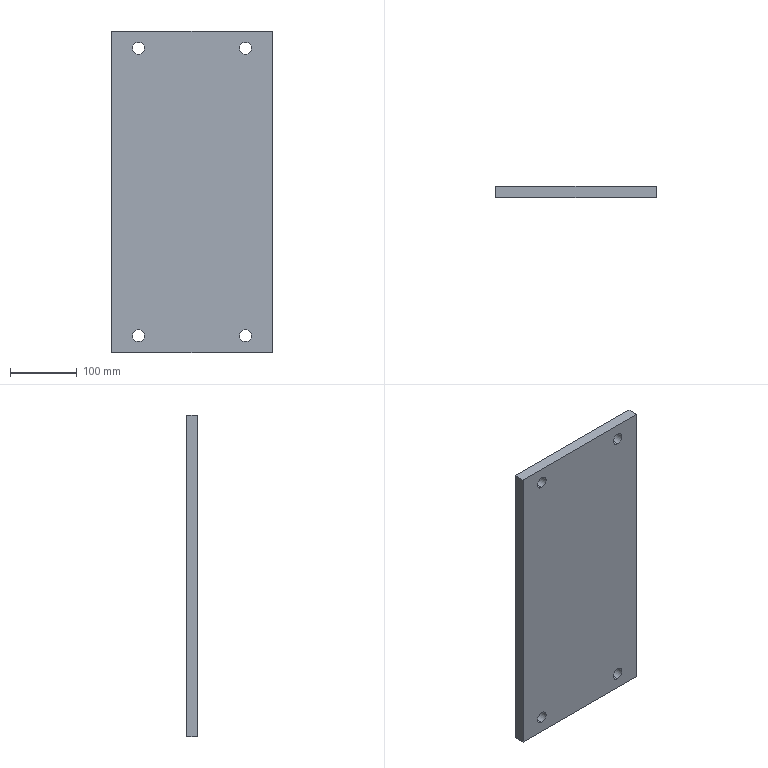Part | SolidWorks | features Chamfer 1, Extrusion 1, Fillet 1, HoleWzd 1 | 1 solid | 14 faces | box 240 x 16 x 480 mm | volume 1826914 mm3 | cylinder 8 | plane 6 | commonest cylinder face diameters 18 x8
STEP:
#1=CARTESIAN_POINT('',(-80.,0.,206.));
#2=VERTEX_POINT('',#1);
#3=CARTESIAN_POINT('',(-80.,0.,224.));
#4=VERTEX_POINT('',#3);
#5=CARTESIAN_POINT('',(-80.,0.,215.));
#6=DIRECTION('',(0.,1.,0.));
#7=DIRECTION('',(0.,0.,1.));
#8=AXIS2_PLACEMENT_3D('',#5,#6,#7);
#9=CIRCLE('',#8,9.);
#10=EDGE_CURVE('',#2,#4,#9,.T.);
#11=ORIENTED_EDGE('',*,*,#10,.F.);
#12=CARTESIAN_POINT('',(-80.,16.,206.));
#13=VERTEX_POINT('',#12);
#14=CARTESIAN_POINT('',(-80.,16.,206.));
#15=DIRECTION('',(0.,1.,0.));
#16=VECTOR('',#15,1000.);
#17=LINE('',#14,#16);
#18=EDGE_CURVE('',#2,#13,#17,.T.);
#19=ORIENTED_EDGE('',*,*,#18,.T.);
#20=CARTESIAN_POINT('',(-80.,16.,224.));
#21=VERTEX_POINT('',#20);
#22=CARTESIAN_POINT('',(-80.,16.,215.));
#23=DIRECTION('',(0.,1.,0.));
#24=DIRECTION('',(0.,0.,1.));
#25=AXIS2_PLACEMENT_3D('',#22,#23,#24);
#26=CIRCLE('',#25,9.);
#27=EDGE_CURVE('',#13,#21,#26,.T.);
#28=ORIENTED_EDGE('',*,*,#27,.T.);
#29=CARTESIAN_POINT('',(-80.,16.,224.));
#30=DIRECTION('',(0.,1.,0.));
#31=VECTOR('',#30,1000.);
#32=LINE('',#29,#31);
#33=EDGE_CURVE('',#4,#21,#32,.T.);
#34=ORIENTED_EDGE('',*,*,#33,.F.);
#35=EDGE_LOOP('',(#11,#19,#28,#34));
#36=FACE_OUTER_BOUND('',#35,.T.);
#37=CARTESIAN_POINT('',(-80.,16.,215.));
#38=DIRECTION('',(0.,1.,0.));
#39=DIRECTION('',(0.,0.,1.));
#40=AXIS2_PLACEMENT_3D('',#37,#38,#39);
#41=CYLINDRICAL_SURFACE('',#40,9.);
#42=ADVANCED_FACE('',(#36),#41,.F.);
#43=CARTESIAN_POINT('',(80.,0.,206.));
#44=VERTEX_POINT('',#43);
#45=CARTESIAN_POINT('',(80.,0.,224.));
#46=VERTEX_POINT('',#45);
#47=CARTESIAN_POINT('',(80.,0.,215.));
#48=DIRECTION('',(0.,1.,0.));
#49=DIRECTION('',(0.,0.,1.));
#50=AXIS2_PLACEMENT_3D('',#47,#48,#49);
#51=CIRCLE('',#50,9.);
#52=EDGE_CURVE('',#44,#46,#51,.T.);
#53=ORIENTED_EDGE('',*,*,#52,.F.);
#54=CARTESIAN_POINT('',(80.,16.,206.));
#55=VERTEX_POINT('',#54);
#56=CARTESIAN_POINT('',(80.,16.,206.));
#57=DIRECTION('',(0.,1.,0.));
#58=VECTOR('',#57,1000.);
#59=LINE('',#56,#58);
#60=EDGE_CURVE('',#44,#55,#59,.T.);
#61=ORIENTED_EDGE('',*,*,#60,.T.);
#62=CARTESIAN_POINT('',(80.,16.,224.));
#63=VERTEX_POINT('',#62);
#64=CARTESIAN_POINT('',(80.,16.,215.));
#65=DIRECTION('',(0.,1.,0.));
#66=DIRECTION('',(0.,0.,1.));
#67=AXIS2_PLACEMENT_3D('',#64,#65,#66);
#68=CIRCLE('',#67,9.);
#69=EDGE_CURVE('',#55,#63,#68,.T.);
#70=ORIENTED_EDGE('',*,*,#69,.T.);
#71=CARTESIAN_POINT('',(80.,16.,224.));
#72=DIRECTION('',(0.,1.,0.));
#73=VECTOR('',#72,1000.);
#74=LINE('',#71,#73);
#75=EDGE_CURVE('',#46,#63,#74,.T.);
#76=ORIENTED_EDGE('',*,*,#75,.F.);
#77=EDGE_LOOP('',(#53,#61,#70,#76));
#78=FACE_OUTER_BOUND('',#77,.T.);
#79=CARTESIAN_POINT('',(80.,16.,215.));
#80=DIRECTION('',(0.,1.,0.));
#81=DIRECTION('',(0.,0.,1.));
#82=AXIS2_PLACEMENT_3D('',#79,#80,#81);
#83=CYLINDRICAL_SURFACE('',#82,9.);
#84=ADVANCED_FACE('',(#78),#83,.F.);
#85=CARTESIAN_POINT('',(80.,0.,-224.));
#86=VERTEX_POINT('',#85);
#87=CARTESIAN_POINT('',(80.,0.,-206.));
#88=VERTEX_POINT('',#87);
#89=CARTESIAN_POINT('',(80.,0.,-215.));
#90=DIRECTION('',(0.,1.,0.));
#91=DIRECTION('',(0.,0.,1.));
#92=AXIS2_PLACEMENT_3D('',#89,#90,#91);
#93=CIRCLE('',#92,9.);
#94=EDGE_CURVE('',#86,#88,#93,.T.);
#95=ORIENTED_EDGE('',*,*,#94,.F.);
#96=CARTESIAN_POINT('',(80.,16.,-224.));
#97=VERTEX_POINT('',#96);
#98=CARTESIAN_POINT('',(80.,16.,-224.));
#99=DIRECTION('',(0.,1.,0.));
#100=VECTOR('',#99,1000.);
#101=LINE('',#98,#100);
#102=EDGE_CURVE('',#86,#97,#101,.T.);
#103=ORIENTED_EDGE('',*,*,#102,.T.);
#104=CARTESIAN_POINT('',(80.,16.,-206.));
#105=VERTEX_POINT('',#104);
#106=CARTESIAN_POINT('',(80.,16.,-215.));
#107=DIRECTION('',(0.,1.,0.));
#108=DIRECTION('',(0.,0.,1.));
#109=AXIS2_PLACEMENT_3D('',#106,#107,#108);
#110=CIRCLE('',#109,9.);
#111=EDGE_CURVE('',#97,#105,#110,.T.);
#112=ORIENTED_EDGE('',*,*,#111,.T.);
#113=CARTESIAN_POINT('',(80.,16.,-206.));
#114=DIRECTION('',(0.,1.,0.));
#115=VECTOR('',#114,1000.);
#116=LINE('',#113,#115);
#117=EDGE_CURVE('',#88,#105,#116,.T.);
#118=ORIENTED_EDGE('',*,*,#117,.F.);
#119=EDGE_LOOP('',(#95,#103,#112,#118));
#120=FACE_OUTER_BOUND('',#119,.T.);
#121=CARTESIAN_POINT('',(80.,16.,-215.));
#122=DIRECTION('',(0.,1.,0.));
#123=DIRECTION('',(0.,0.,1.));
#124=AXIS2_PLACEMENT_3D('',#121,#122,#123);
#125=CYLINDRICAL_SURFACE('',#124,9.);
#126=ADVANCED_FACE('',(#120),#125,.F.);
#127=CARTESIAN_POINT('',(-80.,0.,-224.));
#128=VERTEX_POINT('',#127);
#129=CARTESIAN_POINT('',(-80.,0.,-206.));
#130=VERTEX_POINT('',#129);
#131=CARTESIAN_POINT('',(-80.,0.,-215.));
#132=DIRECTION('',(0.,1.,0.));
#133=DIRECTION('',(0.,0.,1.));
#134=AXIS2_PLACEMENT_3D('',#131,#132,#133);
#135=CIRCLE('',#134,9.);
#136=EDGE_CURVE('',#128,#130,#135,.T.);
#137=ORIENTED_EDGE('',*,*,#136,.F.);
#138=CARTESIAN_POINT('',(-80.,16.,-224.));
#139=VERTEX_POINT('',#138);
#140=CARTESIAN_POINT('',(-80.,16.,-224.));
#141=DIRECTION('',(0.,1.,0.));
#142=VECTOR('',#141,1000.);
#143=LINE('',#140,#142);
#144=EDGE_CURVE('',#128,#139,#143,.T.);
#145=ORIENTED_EDGE('',*,*,#144,.T.);
#146=CARTESIAN_POINT('',(-80.,16.,-206.));
#147=VERTEX_POINT('',#146);
#148=CARTESIAN_POINT('',(-80.,16.,-215.));
#149=DIRECTION('',(0.,1.,0.));
#150=DIRECTION('',(0.,0.,1.));
#151=AXIS2_PLACEMENT_3D('',#148,#149,#150);
#152=CIRCLE('',#151,9.);
#153=EDGE_CURVE('',#139,#147,#152,.T.);
#154=ORIENTED_EDGE('',*,*,#153,.T.);
#155=CARTESIAN_POINT('',(-80.,16.,-206.));
#156=DIRECTION('',(0.,1.,0.));
#157=VECTOR('',#156,1000.);
#158=LINE('',#155,#157);
#159=EDGE_CURVE('',#130,#147,#158,.T.);
#160=ORIENTED_EDGE('',*,*,#159,.F.);
#161=EDGE_LOOP('',(#137,#145,#154,#160));
#162=FACE_OUTER_BOUND('',#161,.T.);
#163=CARTESIAN_POINT('',(-80.,16.,-215.));
#164=DIRECTION('',(0.,1.,0.));
#165=DIRECTION('',(0.,0.,1.));
#166=AXIS2_PLACEMENT_3D('',#163,#164,#165);
#167=CYLINDRICAL_SURFACE('',#166,9.);
#168=ADVANCED_FACE('',(#162),#167,.F.);
#169=CARTESIAN_POINT('',(-120.,0.,-240.));
#170=VERTEX_POINT('',#169);
#171=CARTESIAN_POINT('',(-120.,0.,240.));
#172=VERTEX_POINT('',#171);
#173=CARTESIAN_POINT('',(-120.,0.,240.));
#174=DIRECTION('',(0.,0.,1.));
#175=VECTOR('',#174,1000.);
#176=LINE('',#173,#175);
#177=EDGE_CURVE('',#170,#172,#176,.T.);
#178=ORIENTED_EDGE('',*,*,#177,.T.);
#179=CARTESIAN_POINT('',(-120.,16.,240.));
#180=VERTEX_POINT('',#179);
#181=CARTESIAN_POINT('',(-120.,16.,240.));
#182=DIRECTION('',(0.,-1.,0.));
#183=VECTOR('',#182,1000.);
#184=LINE('',#181,#183);
#185=EDGE_CURVE('',#180,#172,#184,.T.);
#186=ORIENTED_EDGE('',*,*,#185,.F.);
#187=CARTESIAN_POINT('',(-120.,16.,-240.));
#188=VERTEX_POINT('',#187);
#189=CARTESIAN_POINT('',(-120.,16.,240.));
#190=DIRECTION('',(0.,0.,1.));
#191=VECTOR('',#190,1000.);
#192=LINE('',#189,#191);
#193=EDGE_CURVE('',#188,#180,#192,.T.);
#194=ORIENTED_EDGE('',*,*,#193,.F.);
#195=CARTESIAN_POINT('',(-120.,16.,-240.));
#196=DIRECTION('',(0.,-1.,0.));
#197=VECTOR('',#196,1000.);
#198=LINE('',#195,#197);
#199=EDGE_CURVE('',#188,#170,#198,.T.);
#200=ORIENTED_EDGE('',*,*,#199,.T.);
#201=EDGE_LOOP('',(#178,#186,#194,#200));
#202=FACE_OUTER_BOUND('',#201,.T.);
#203=CARTESIAN_POINT('',(-120.,16.,240.));
#204=DIRECTION('',(1.,0.,0.));
#205=DIRECTION('',(0.,0.,-1.));
#206=AXIS2_PLACEMENT_3D('',#203,#204,#205);
#207=PLANE('',#206);
#208=ADVANCED_FACE('',(#202),#207,.F.);
#209=CARTESIAN_POINT('',(120.,0.,240.));
#210=VERTEX_POINT('',#209);
#211=CARTESIAN_POINT('',(120.,0.,240.));
#212=DIRECTION('',(1.,0.,0.));
#213=VECTOR('',#212,1000.);
#214=LINE('',#211,#213);
#215=EDGE_CURVE('',#172,#210,#214,.T.);
#216=ORIENTED_EDGE('',*,*,#215,.T.);
#217=CARTESIAN_POINT('',(120.,16.,240.));
#218=VERTEX_POINT('',#217);
#219=CARTESIAN_POINT('',(120.,16.,240.));
#220=DIRECTION('',(0.,-1.,0.));
#221=VECTOR('',#220,1000.);
#222=LINE('',#219,#221);
#223=EDGE_CURVE('',#218,#210,#222,.T.);
#224=ORIENTED_EDGE('',*,*,#223,.F.);
#225=CARTESIAN_POINT('',(120.,16.,240.));
#226=DIRECTION('',(1.,0.,0.));
#227=VECTOR('',#226,1000.);
#228=LINE('',#225,#227);
#229=EDGE_CURVE('',#180,#218,#228,.T.);
#230=ORIENTED_EDGE('',*,*,#229,.F.);
#231=ORIENTED_EDGE('',*,*,#185,.T.);
#232=EDGE_LOOP('',(#216,#224,#230,#231));
#233=FACE_OUTER_BOUND('',#232,.T.);
#234=CARTESIAN_POINT('',(120.,16.,240.));
#235=DIRECTION('',(0.,0.,-1.));
#236=DIRECTION('',(-1.,0.,0.));
#237=AXIS2_PLACEMENT_3D('',#234,#235,#236);
#238=PLANE('',#237);
#239=ADVANCED_FACE('',(#233),#238,.F.);
#240=CARTESIAN_POINT('',(120.,0.,-240.));
#241=VERTEX_POINT('',#240);
#242=CARTESIAN_POINT('',(120.,0.,240.));
#243=DIRECTION('',(0.,0.,-1.));
#244=VECTOR('',#243,1000.);
#245=LINE('',#242,#244);
#246=EDGE_CURVE('',#210,#241,#245,.T.);
#247=ORIENTED_EDGE('',*,*,#246,.T.);
#248=CARTESIAN_POINT('',(120.,16.,-240.));
#249=VERTEX_POINT('',#248);
#250=CARTESIAN_POINT('',(120.,16.,-240.));
#251=DIRECTION('',(0.,-1.,0.));
#252=VECTOR('',#251,1000.);
#253=LINE('',#250,#252);
#254=EDGE_CURVE('',#249,#241,#253,.T.);
#255=ORIENTED_EDGE('',*,*,#254,.F.);
#256=CARTESIAN_POINT('',(120.,16.,240.));
#257=DIRECTION('',(0.,0.,-1.));
#258=VECTOR('',#257,1000.);
#259=LINE('',#256,#258);
#260=EDGE_CURVE('',#218,#249,#259,.T.);
#261=ORIENTED_EDGE('',*,*,#260,.F.);
#262=ORIENTED_EDGE('',*,*,#223,.T.);
#263=EDGE_LOOP('',(#247,#255,#261,#262));
#264=FACE_OUTER_BOUND('',#263,.T.);
#265=CARTESIAN_POINT('',(120.,16.,240.));
#266=DIRECTION('',(-1.,0.,0.));
#267=DIRECTION('',(0.,0.,1.));
#268=AXIS2_PLACEMENT_3D('',#265,#266,#267);
#269=PLANE('',#268);
#270=ADVANCED_FACE('',(#264),#269,.F.);
#271=CARTESIAN_POINT('',(120.,0.,-240.));
#272=DIRECTION('',(-1.,0.,0.));
#273=VECTOR('',#272,1000.);
#274=LINE('',#271,#273);
#275=EDGE_CURVE('',#241,#170,#274,.T.);
#276=ORIENTED_EDGE('',*,*,#275,.T.);
#277=ORIENTED_EDGE('',*,*,#199,.F.);
#278=CARTESIAN_POINT('',(120.,16.,-240.));
#279=DIRECTION('',(-1.,0.,0.));
#280=VECTOR('',#279,1000.);
#281=LINE('',#278,#280);
#282=EDGE_CURVE('',#249,#188,#281,.T.);
#283=ORIENTED_EDGE('',*,*,#282,.F.);
#284=ORIENTED_EDGE('',*,*,#254,.T.);
#285=EDGE_LOOP('',(#276,#277,#283,#284));
#286=FACE_OUTER_BOUND('',#285,.T.);
#287=CARTESIAN_POINT('',(120.,16.,-240.));
#288=DIRECTION('',(0.,0.,1.));
#289=DIRECTION('',(1.,0.,0.));
#290=AXIS2_PLACEMENT_3D('',#287,#288,#289);
#291=PLANE('',#290);
#292=ADVANCED_FACE('',(#286),#291,.F.);
#293=CARTESIAN_POINT('',(-80.,16.,215.));
#294=DIRECTION('',(0.,1.,0.));
#295=DIRECTION('',(0.,0.,1.));
#296=AXIS2_PLACEMENT_3D('',#293,#294,#295);
#297=CIRCLE('',#296,9.);
#298=EDGE_CURVE('',#21,#13,#297,.T.);
#299=ORIENTED_EDGE('',*,*,#298,.F.);
#300=ORIENTED_EDGE('',*,*,#27,.F.);
#301=EDGE_LOOP('',(#299,#300));
#302=FACE_BOUND('',#301,.T.);
#303=CARTESIAN_POINT('',(80.,16.,215.));
#304=DIRECTION('',(0.,1.,0.));
#305=DIRECTION('',(0.,0.,1.));
#306=AXIS2_PLACEMENT_3D('',#303,#304,#305);
#307=CIRCLE('',#306,9.);
#308=EDGE_CURVE('',#63,#55,#307,.T.);
#309=ORIENTED_EDGE('',*,*,#308,.F.);
#310=ORIENTED_EDGE('',*,*,#69,.F.);
#311=EDGE_LOOP('',(#309,#310));
#312=FACE_BOUND('',#311,.T.);
#313=CARTESIAN_POINT('',(80.,16.,-215.));
#314=DIRECTION('',(0.,1.,0.));
#315=DIRECTION('',(0.,0.,1.));
#316=AXIS2_PLACEMENT_3D('',#313,#314,#315);
#317=CIRCLE('',#316,9.);
#318=EDGE_CURVE('',#105,#97,#317,.T.);
#319=ORIENTED_EDGE('',*,*,#318,.F.);
#320=ORIENTED_EDGE('',*,*,#111,.F.);
#321=EDGE_LOOP('',(#319,#320));
#322=FACE_BOUND('',#321,.T.);
#323=CARTESIAN_POINT('',(-80.,16.,-215.));
#324=DIRECTION('',(0.,1.,0.));
#325=DIRECTION('',(0.,0.,1.));
#326=AXIS2_PLACEMENT_3D('',#323,#324,#325);
#327=CIRCLE('',#326,9.);
#328=EDGE_CURVE('',#147,#139,#327,.T.);
#329=ORIENTED_EDGE('',*,*,#328,.F.);
#330=ORIENTED_EDGE('',*,*,#153,.F.);
#331=EDGE_LOOP('',(#329,#330));
#332=FACE_BOUND('',#331,.T.);
#333=ORIENTED_EDGE('',*,*,#193,.T.);
#334=ORIENTED_EDGE('',*,*,#229,.T.);
#335=ORIENTED_EDGE('',*,*,#260,.T.);
#336=ORIENTED_EDGE('',*,*,#282,.T.);
#337=EDGE_LOOP('',(#333,#334,#335,#336));
#338=FACE_OUTER_BOUND('',#337,.T.);
#339=CARTESIAN_POINT('',(0.,16.,0.));
#340=DIRECTION('',(0.,1.,0.));
#341=DIRECTION('',(0.,0.,1.));
#342=AXIS2_PLACEMENT_3D('',#339,#340,#341);
#343=PLANE('',#342);
#344=ADVANCED_FACE('',(#302,#312,#322,#332,#338),#343,.T.);
#345=CARTESIAN_POINT('',(-80.,0.,215.));
#346=DIRECTION('',(0.,1.,0.));
#347=DIRECTION('',(0.,0.,1.));
#348=AXIS2_PLACEMENT_3D('',#345,#346,#347);
#349=CIRCLE('',#348,9.);
#350=EDGE_CURVE('',#4,#2,#349,.T.);
#351=ORIENTED_EDGE('',*,*,#350,.T.);
#352=ORIENTED_EDGE('',*,*,#10,.T.);
#353=EDGE_LOOP('',(#351,#352));
#354=FACE_BOUND('',#353,.T.);
#355=CARTESIAN_POINT('',(80.,0.,215.));
#356=DIRECTION('',(0.,1.,0.));
#357=DIRECTION('',(0.,0.,1.));
#358=AXIS2_PLACEMENT_3D('',#355,#356,#357);
#359=CIRCLE('',#358,9.);
#360=EDGE_CURVE('',#46,#44,#359,.T.);
#361=ORIENTED_EDGE('',*,*,#360,.T.);
#362=ORIENTED_EDGE('',*,*,#52,.T.);
#363=EDGE_LOOP('',(#361,#362));
#364=FACE_BOUND('',#363,.T.);
#365=CARTESIAN_POINT('',(80.,0.,-215.));
#366=DIRECTION('',(0.,1.,0.));
#367=DIRECTION('',(0.,0.,1.));
#368=AXIS2_PLACEMENT_3D('',#365,#366,#367);
#369=CIRCLE('',#368,9.);
#370=EDGE_CURVE('',#88,#86,#369,.T.);
#371=ORIENTED_EDGE('',*,*,#370,.T.);
#372=ORIENTED_EDGE('',*,*,#94,.T.);
#373=EDGE_LOOP('',(#371,#372));
#374=FACE_BOUND('',#373,.T.);
#375=CARTESIAN_POINT('',(-80.,0.,-215.));
#376=DIRECTION('',(0.,1.,0.));
#377=DIRECTION('',(0.,0.,1.));
#378=AXIS2_PLACEMENT_3D('',#375,#376,#377);
#379=CIRCLE('',#378,9.);
#380=EDGE_CURVE('',#130,#128,#379,.T.);
#381=ORIENTED_EDGE('',*,*,#380,.T.);
#382=ORIENTED_EDGE('',*,*,#136,.T.);
#383=EDGE_LOOP('',(#381,#382));
#384=FACE_BOUND('',#383,.T.);
#385=ORIENTED_EDGE('',*,*,#177,.F.);
#386=ORIENTED_EDGE('',*,*,#275,.F.);
#387=ORIENTED_EDGE('',*,*,#246,.F.);
#388=ORIENTED_EDGE('',*,*,#215,.F.);
#389=EDGE_LOOP('',(#385,#386,#387,#388));
#390=FACE_OUTER_BOUND('',#389,.T.);
#391=CARTESIAN_POINT('',(0.,0.,0.));
#392=DIRECTION('',(0.,1.,0.));
#393=DIRECTION('',(0.,0.,1.));
#394=AXIS2_PLACEMENT_3D('',#391,#392,#393);
#395=PLANE('',#394);
#396=ADVANCED_FACE('',(#354,#364,#374,#384,#390),#395,.F.);
#397=ORIENTED_EDGE('',*,*,#144,.F.);
#398=ORIENTED_EDGE('',*,*,#380,.F.);
#399=ORIENTED_EDGE('',*,*,#159,.T.);
#400=ORIENTED_EDGE('',*,*,#328,.T.);
#401=EDGE_LOOP('',(#397,#398,#399,#400));
#402=FACE_OUTER_BOUND('',#401,.T.);
#403=CARTESIAN_POINT('',(-80.,16.,-215.));
#404=DIRECTION('',(0.,1.,0.));
#405=DIRECTION('',(0.,0.,1.));
#406=AXIS2_PLACEMENT_3D('',#403,#404,#405);
#407=CYLINDRICAL_SURFACE('',#406,9.);
#408=ADVANCED_FACE('',(#402),#407,.F.);
#409=ORIENTED_EDGE('',*,*,#102,.F.);
#410=ORIENTED_EDGE('',*,*,#370,.F.);
#411=ORIENTED_EDGE('',*,*,#117,.T.);
#412=ORIENTED_EDGE('',*,*,#318,.T.);
#413=EDGE_LOOP('',(#409,#410,#411,#412));
#414=FACE_OUTER_BOUND('',#413,.T.);
#415=CARTESIAN_POINT('',(80.,16.,-215.));
#416=DIRECTION('',(0.,1.,0.));
#417=DIRECTION('',(0.,0.,1.));
#418=AXIS2_PLACEMENT_3D('',#415,#416,#417);
#419=CYLINDRICAL_SURFACE('',#418,9.);
#420=ADVANCED_FACE('',(#414),#419,.F.);
#421=ORIENTED_EDGE('',*,*,#60,.F.);
#422=ORIENTED_EDGE('',*,*,#360,.F.);
#423=ORIENTED_EDGE('',*,*,#75,.T.);
#424=ORIENTED_EDGE('',*,*,#308,.T.);
#425=EDGE_LOOP('',(#421,#422,#423,#424));
#426=FACE_OUTER_BOUND('',#425,.T.);
#427=CARTESIAN_POINT('',(80.,16.,215.));
#428=DIRECTION('',(0.,1.,0.));
#429=DIRECTION('',(0.,0.,1.));
#430=AXIS2_PLACEMENT_3D('',#427,#428,#429);
#431=CYLINDRICAL_SURFACE('',#430,9.);
#432=ADVANCED_FACE('',(#426),#431,.F.);
#433=ORIENTED_EDGE('',*,*,#18,.F.);
#434=ORIENTED_EDGE('',*,*,#350,.F.);
#435=ORIENTED_EDGE('',*,*,#33,.T.);
#436=ORIENTED_EDGE('',*,*,#298,.T.);
#437=EDGE_LOOP('',(#433,#434,#435,#436));
#438=FACE_OUTER_BOUND('',#437,.T.);
#439=CARTESIAN_POINT('',(-80.,16.,215.));
#440=DIRECTION('',(0.,1.,0.));
#441=DIRECTION('',(0.,0.,1.));
#442=AXIS2_PLACEMENT_3D('',#439,#440,#441);
#443=CYLINDRICAL_SURFACE('',#442,9.);
#444=ADVANCED_FACE('',(#438),#443,.F.);
#445=CLOSED_SHELL('',(#42,#84,#126,#168,#208,#239,#270,#292,#344,#396,#408,#420,#432,#444));
#446=MANIFOLD_SOLID_BREP('',#445);
#447=CARTESIAN_POINT('',(0.,0.,0.));
#448=DIRECTION('',(0.,0.,1.));
#449=DIRECTION('',(1.,0.,0.));
#450=AXIS2_PLACEMENT_3D('',#447,#448,#449);
#451=(LENGTH_UNIT()NAMED_UNIT(*)SI_UNIT(.MILLI.,.METRE.));
#452=UNCERTAINTY_MEASURE_WITH_UNIT(LENGTH_MEASURE(0.00001),#451,'','');
#453=(NAMED_UNIT(*)PLANE_ANGLE_UNIT()SI_UNIT($,.RADIAN.));
#454=(NAMED_UNIT(*)SI_UNIT($,.STERADIAN.)SOLID_ANGLE_UNIT());
#455=(GEOMETRIC_REPRESENTATION_CONTEXT(3)GLOBAL_UNCERTAINTY_ASSIGNED_CONTEXT((#452))GLOBAL_UNIT_ASSIGNED_CONTEXT((#451,#453,#454))REPRESENTATION_CONTEXT('',''));
#456=ADVANCED_BREP_SHAPE_REPRESENTATION('',(#446,#450),#455);